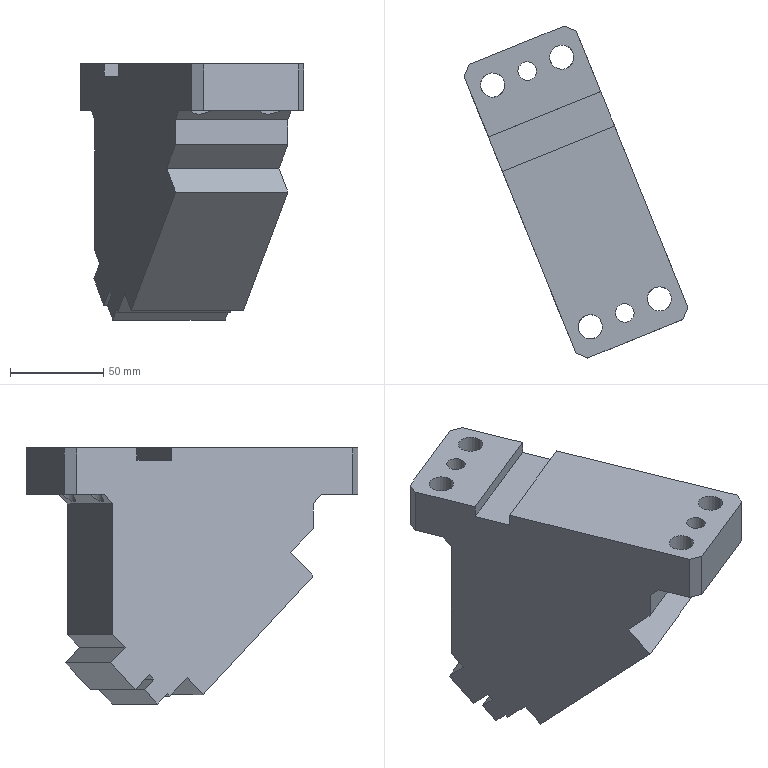Part | NX | features solid 2 | 1 solid | 47 faces | box 120.204 x 178.225 x 137.53 mm | volume 892519 mm3 | plane 37 | cylinder 10 | commonest cylinder face diameters 13 x4 20 x4 10 x2
STEP:
#1=CARTESIAN_POINT('',(-779.548,445.031,38.127));
#2=VERTEX_POINT('',#1);
#3=CARTESIAN_POINT('',(-719.281,469.38,38.127));
#4=VERTEX_POINT('',#3);
#5=CARTESIAN_POINT('',(-779.548,445.031,38.127));
#6=DIRECTION('',(0.9272,0.3746,0.));
#7=VECTOR('',#6,1000.);
#8=LINE('',#5,#7);
#9=EDGE_CURVE('',#2,#4,#8,.T.);
#10=ORIENTED_EDGE('',*,*,#9,.T.);
#11=CARTESIAN_POINT('',(-718.752,468.069,36.712));
#12=VERTEX_POINT('',#11);
#13=CARTESIAN_POINT('',(-731.128,498.702,69.751));
#14=DIRECTION('',(0.2649,-0.6556,-0.7071));
#15=VECTOR('',#14,1000.);
#16=LINE('',#13,#15);
#17=EDGE_CURVE('',#4,#12,#16,.T.);
#18=ORIENTED_EDGE('',*,*,#17,.T.);
#19=CARTESIAN_POINT('',(-779.018,443.719,36.712));
#20=VERTEX_POINT('',#19);
#21=CARTESIAN_POINT('',(-779.018,443.719,36.712));
#22=DIRECTION('',(0.9272,0.3746,0.));
#23=VECTOR('',#22,1000.);
#24=LINE('',#21,#23);
#25=EDGE_CURVE('',#20,#12,#24,.T.);
#26=ORIENTED_EDGE('',*,*,#25,.F.);
#27=CARTESIAN_POINT('',(-791.395,474.352,69.751));
#28=DIRECTION('',(0.2649,-0.6556,-0.7071));
#29=VECTOR('',#28,1000.);
#30=LINE('',#27,#29);
#31=EDGE_CURVE('',#2,#20,#30,.T.);
#32=ORIENTED_EDGE('',*,*,#31,.F.);
#33=EDGE_LOOP('',(#10,#18,#26,#32));
#34=FACE_BOUND('',#33,.T.);
#35=CARTESIAN_POINT('',(-791.395,474.352,69.751));
#36=DIRECTION('',(-0.2649,0.6556,-0.7071));
#37=DIRECTION('',(0.2649,-0.6556,-0.7071));
#38=AXIS2_PLACEMENT_3D('',#35,#36,#37);
#39=PLANE('',#38);
#40=ADVANCED_FACE('',(#34),#39,.T.);
#41=CARTESIAN_POINT('',(-791.395,474.352,69.751));
#42=VERTEX_POINT('',#41);
#43=CARTESIAN_POINT('',(-788.746,467.796,62.68));
#44=VERTEX_POINT('',#43);
#45=CARTESIAN_POINT('',(-791.395,474.352,69.751));
#46=DIRECTION('',(0.2649,-0.6556,-0.7071));
#47=VECTOR('',#46,1000.);
#48=LINE('',#45,#47);
#49=EDGE_CURVE('',#42,#44,#48,.T.);
#50=ORIENTED_EDGE('',*,*,#49,.F.);
#51=CARTESIAN_POINT('',(-731.128,498.702,69.751));
#52=VERTEX_POINT('',#51);
#53=CARTESIAN_POINT('',(-791.395,474.352,69.751));
#54=DIRECTION('',(0.9272,0.3746,0.));
#55=VECTOR('',#54,1000.);
#56=LINE('',#53,#55);
#57=EDGE_CURVE('',#42,#52,#56,.T.);
#58=ORIENTED_EDGE('',*,*,#57,.T.);
#59=CARTESIAN_POINT('',(-728.479,492.145,62.68));
#60=VERTEX_POINT('',#59);
#61=CARTESIAN_POINT('',(-731.128,498.702,69.751));
#62=DIRECTION('',(0.2649,-0.6556,-0.7071));
#63=VECTOR('',#62,1000.);
#64=LINE('',#61,#63);
#65=EDGE_CURVE('',#52,#60,#64,.T.);
#66=ORIENTED_EDGE('',*,*,#65,.T.);
#67=CARTESIAN_POINT('',(-788.746,467.796,62.68));
#68=DIRECTION('',(0.9272,0.3746,0.));
#69=VECTOR('',#68,1000.);
#70=LINE('',#67,#69);
#71=EDGE_CURVE('',#44,#60,#70,.T.);
#72=ORIENTED_EDGE('',*,*,#71,.F.);
#73=EDGE_LOOP('',(#50,#58,#66,#72));
#74=FACE_BOUND('',#73,.T.);
#75=CARTESIAN_POINT('',(-791.395,474.352,69.751));
#76=DIRECTION('',(-0.2649,0.6556,-0.7071));
#77=DIRECTION('',(0.2649,-0.6556,-0.7071));
#78=AXIS2_PLACEMENT_3D('',#75,#76,#77);
#79=PLANE('',#78);
#80=ADVANCED_FACE('',(#74),#79,.T.);
#81=CARTESIAN_POINT('',(-782.462,452.243,45.905));
#82=VERTEX_POINT('',#81);
#83=CARTESIAN_POINT('',(-722.195,476.592,45.905));
#84=VERTEX_POINT('',#83);
#85=CARTESIAN_POINT('',(-782.462,452.243,45.905));
#86=DIRECTION('',(0.9272,0.3746,0.));
#87=VECTOR('',#86,1000.);
#88=LINE('',#85,#87);
#89=EDGE_CURVE('',#82,#84,#88,.T.);
#90=ORIENTED_EDGE('',*,*,#89,.F.);
#91=CARTESIAN_POINT('',(-783.448,454.684,48.538));
#92=VERTEX_POINT('',#91);
#93=CARTESIAN_POINT('',(-791.395,474.352,69.751));
#94=DIRECTION('',(0.2649,-0.6556,-0.7071));
#95=VECTOR('',#94,1000.);
#96=LINE('',#93,#95);
#97=EDGE_CURVE('',#92,#82,#96,.T.);
#98=ORIENTED_EDGE('',*,*,#97,.F.);
#99=CARTESIAN_POINT('',(-723.181,479.033,48.538));
#100=VERTEX_POINT('',#99);
#101=CARTESIAN_POINT('',(-783.448,454.684,48.538));
#102=DIRECTION('',(0.9272,0.3746,0.));
#103=VECTOR('',#102,1000.);
#104=LINE('',#101,#103);
#105=EDGE_CURVE('',#92,#100,#104,.T.);
#106=ORIENTED_EDGE('',*,*,#105,.T.);
#107=CARTESIAN_POINT('',(-731.128,498.702,69.751));
#108=DIRECTION('',(0.2649,-0.6556,-0.7071));
#109=VECTOR('',#108,1000.);
#110=LINE('',#107,#109);
#111=EDGE_CURVE('',#100,#84,#110,.T.);
#112=ORIENTED_EDGE('',*,*,#111,.T.);
#113=EDGE_LOOP('',(#90,#98,#106,#112));
#114=FACE_BOUND('',#113,.T.);
#115=CARTESIAN_POINT('',(-791.395,474.352,69.751));
#116=DIRECTION('',(-0.2649,0.6556,-0.7071));
#117=DIRECTION('',(0.2649,-0.6556,-0.7071));
#118=AXIS2_PLACEMENT_3D('',#115,#116,#117);
#119=PLANE('',#118);
#120=ADVANCED_FACE('',(#114),#119,.T.);
#121=CARTESIAN_POINT('',(-714.987,458.751,46.763));
#122=VERTEX_POINT('',#121);
#123=CARTESIAN_POINT('',(-718.752,468.069,36.712));
#124=DIRECTION('',(0.2649,-0.6556,0.7071));
#125=VECTOR('',#124,1000.);
#126=LINE('',#123,#125);
#127=EDGE_CURVE('',#12,#122,#126,.T.);
#128=ORIENTED_EDGE('',*,*,#127,.T.);
#129=CARTESIAN_POINT('',(-775.254,434.401,46.763));
#130=VERTEX_POINT('',#129);
#131=CARTESIAN_POINT('',(-775.254,434.401,46.763));
#132=DIRECTION('',(0.9272,0.3746,0.));
#133=VECTOR('',#132,1000.);
#134=LINE('',#131,#133);
#135=EDGE_CURVE('',#130,#122,#134,.T.);
#136=ORIENTED_EDGE('',*,*,#135,.F.);
#137=CARTESIAN_POINT('',(-779.018,443.719,36.712));
#138=DIRECTION('',(0.2649,-0.6556,0.7071));
#139=VECTOR('',#138,1000.);
#140=LINE('',#137,#139);
#141=EDGE_CURVE('',#20,#130,#140,.T.);
#142=ORIENTED_EDGE('',*,*,#141,.F.);
#143=ORIENTED_EDGE('',*,*,#25,.T.);
#144=EDGE_LOOP('',(#128,#136,#142,#143));
#145=FACE_BOUND('',#144,.T.);
#146=CARTESIAN_POINT('',(-779.018,443.719,36.712));
#147=DIRECTION('',(0.2649,-0.6556,-0.7071));
#148=DIRECTION('',(0.2649,-0.6556,0.7071));
#149=AXIS2_PLACEMENT_3D('',#146,#147,#148);
#150=PLANE('',#149);
#151=ADVANCED_FACE('',(#145),#150,.T.);
#152=CARTESIAN_POINT('',(-711.543,450.228,37.57));
#153=VERTEX_POINT('',#152);
#154=CARTESIAN_POINT('',(-714.987,458.751,46.763));
#155=DIRECTION('',(0.2649,-0.6556,-0.7071));
#156=VECTOR('',#155,1000.);
#157=LINE('',#154,#156);
#158=EDGE_CURVE('',#122,#153,#157,.T.);
#159=ORIENTED_EDGE('',*,*,#158,.T.);
#160=CARTESIAN_POINT('',(-771.81,425.878,37.57));
#161=VERTEX_POINT('',#160);
#162=CARTESIAN_POINT('',(-771.81,425.878,37.57));
#163=DIRECTION('',(0.9272,0.3746,0.));
#164=VECTOR('',#163,1000.);
#165=LINE('',#162,#164);
#166=EDGE_CURVE('',#161,#153,#165,.T.);
#167=ORIENTED_EDGE('',*,*,#166,.F.);
#168=CARTESIAN_POINT('',(-775.254,434.401,46.763));
#169=DIRECTION('',(0.2649,-0.6556,-0.7071));
#170=VECTOR('',#169,1000.);
#171=LINE('',#168,#170);
#172=EDGE_CURVE('',#130,#161,#171,.T.);
#173=ORIENTED_EDGE('',*,*,#172,.F.);
#174=ORIENTED_EDGE('',*,*,#135,.T.);
#175=EDGE_LOOP('',(#159,#167,#173,#174));
#176=FACE_BOUND('',#175,.T.);
#177=CARTESIAN_POINT('',(-775.254,434.401,46.763));
#178=DIRECTION('',(-0.2649,0.6556,-0.7071));
#179=DIRECTION('',(0.2649,-0.6556,-0.7071));
#180=AXIS2_PLACEMENT_3D('',#177,#178,#179);
#181=PLANE('',#180);
#182=ADVANCED_FACE('',(#176),#181,.T.);
#183=CARTESIAN_POINT('',(-687.703,391.222,101.21));
#184=VERTEX_POINT('',#183);
#185=CARTESIAN_POINT('',(-711.543,450.228,37.57));
#186=DIRECTION('',(0.2649,-0.6556,0.7071));
#187=VECTOR('',#186,1000.);
#188=LINE('',#185,#187);
#189=EDGE_CURVE('',#153,#184,#188,.T.);
#190=ORIENTED_EDGE('',*,*,#189,.T.);
#191=CARTESIAN_POINT('',(-747.97,366.873,101.21));
#192=VERTEX_POINT('',#191);
#193=CARTESIAN_POINT('',(-747.97,366.873,101.21));
#194=DIRECTION('',(0.9272,0.3746,0.));
#195=VECTOR('',#194,1000.);
#196=LINE('',#193,#195);
#197=EDGE_CURVE('',#192,#184,#196,.T.);
#198=ORIENTED_EDGE('',*,*,#197,.F.);
#199=CARTESIAN_POINT('',(-771.81,425.878,37.57));
#200=DIRECTION('',(0.2649,-0.6556,0.7071));
#201=VECTOR('',#200,1000.);
#202=LINE('',#199,#201);
#203=EDGE_CURVE('',#161,#192,#202,.T.);
#204=ORIENTED_EDGE('',*,*,#203,.F.);
#205=ORIENTED_EDGE('',*,*,#166,.T.);
#206=EDGE_LOOP('',(#190,#198,#204,#205));
#207=FACE_BOUND('',#206,.T.);
#208=CARTESIAN_POINT('',(-771.81,425.878,37.57));
#209=DIRECTION('',(0.2649,-0.6556,-0.7071));
#210=DIRECTION('',(0.2649,-0.6556,0.7071));
#211=AXIS2_PLACEMENT_3D('',#208,#209,#210);
#212=PLANE('',#211);
#213=ADVANCED_FACE('',(#207),#212,.T.);
#214=CARTESIAN_POINT('',(-692.471,403.023,113.938));
#215=VERTEX_POINT('',#214);
#216=CARTESIAN_POINT('',(-692.471,403.023,113.938));
#217=DIRECTION('',(0.2649,-0.6556,-0.7071));
#218=VECTOR('',#217,1000.);
#219=LINE('',#216,#218);
#220=EDGE_CURVE('',#215,#184,#219,.T.);
#221=ORIENTED_EDGE('',*,*,#220,.F.);
#222=CARTESIAN_POINT('',(-752.738,378.674,113.938));
#223=VERTEX_POINT('',#222);
#224=CARTESIAN_POINT('',(-752.738,378.674,113.938));
#225=DIRECTION('',(0.9272,0.3746,0.));
#226=VECTOR('',#225,1000.);
#227=LINE('',#224,#226);
#228=EDGE_CURVE('',#223,#215,#227,.T.);
#229=ORIENTED_EDGE('',*,*,#228,.F.);
#230=CARTESIAN_POINT('',(-752.738,378.674,113.938));
#231=DIRECTION('',(0.2649,-0.6556,-0.7071));
#232=VECTOR('',#231,1000.);
#233=LINE('',#230,#232);
#234=EDGE_CURVE('',#223,#192,#233,.T.);
#235=ORIENTED_EDGE('',*,*,#234,.T.);
#236=ORIENTED_EDGE('',*,*,#197,.T.);
#237=EDGE_LOOP('',(#221,#229,#235,#236));
#238=FACE_BOUND('',#237,.T.);
#239=CARTESIAN_POINT('',(-752.738,378.674,113.938));
#240=DIRECTION('',(-0.2649,0.6556,-0.7071));
#241=DIRECTION('',(0.2649,-0.6556,-0.7071));
#242=AXIS2_PLACEMENT_3D('',#239,#240,#241);
#243=PLANE('',#242);
#244=ADVANCED_FACE('',(#238),#243,.F.);
#245=CARTESIAN_POINT('',(-687.674,391.148,126.745));
#246=VERTEX_POINT('',#245);
#247=CARTESIAN_POINT('',(-692.471,403.023,113.938));
#248=DIRECTION('',(0.2649,-0.6556,0.7071));
#249=VECTOR('',#248,1000.);
#250=LINE('',#247,#249);
#251=EDGE_CURVE('',#215,#246,#250,.T.);
#252=ORIENTED_EDGE('',*,*,#251,.T.);
#253=CARTESIAN_POINT('',(-747.941,366.799,126.745));
#254=VERTEX_POINT('',#253);
#255=CARTESIAN_POINT('',(-747.941,366.799,126.745));
#256=DIRECTION('',(0.9272,0.3746,0.));
#257=VECTOR('',#256,1000.);
#258=LINE('',#255,#257);
#259=EDGE_CURVE('',#254,#246,#258,.T.);
#260=ORIENTED_EDGE('',*,*,#259,.F.);
#261=CARTESIAN_POINT('',(-752.738,378.674,113.938));
#262=DIRECTION('',(0.2649,-0.6556,0.7071));
#263=VECTOR('',#262,1000.);
#264=LINE('',#261,#263);
#265=EDGE_CURVE('',#223,#254,#264,.T.);
#266=ORIENTED_EDGE('',*,*,#265,.F.);
#267=ORIENTED_EDGE('',*,*,#228,.T.);
#268=EDGE_LOOP('',(#252,#260,#266,#267));
#269=FACE_BOUND('',#268,.T.);
#270=CARTESIAN_POINT('',(-752.738,378.674,113.938));
#271=DIRECTION('',(0.2649,-0.6556,-0.7071));
#272=DIRECTION('',(0.2649,-0.6556,0.7071));
#273=AXIS2_PLACEMENT_3D('',#270,#271,#272);
#274=PLANE('',#273);
#275=ADVANCED_FACE('',(#269),#274,.T.);
#276=CARTESIAN_POINT('',(-747.941,366.799,140.));
#277=VERTEX_POINT('',#276);
#278=CARTESIAN_POINT('',(-747.941,366.799,145.));
#279=DIRECTION('',(0.,0.,-1.));
#280=VECTOR('',#279,1000.);
#281=LINE('',#278,#280);
#282=EDGE_CURVE('',#277,#254,#281,.T.);
#283=ORIENTED_EDGE('',*,*,#282,.T.);
#284=ORIENTED_EDGE('',*,*,#259,.T.);
#285=CARTESIAN_POINT('',(-687.674,391.148,140.));
#286=VERTEX_POINT('',#285);
#287=CARTESIAN_POINT('',(-687.674,391.148,145.));
#288=DIRECTION('',(0.,0.,-1.));
#289=VECTOR('',#288,1000.);
#290=LINE('',#287,#289);
#291=EDGE_CURVE('',#286,#246,#290,.T.);
#292=ORIENTED_EDGE('',*,*,#291,.F.);
#293=CARTESIAN_POINT('',(-747.941,366.799,140.));
#294=DIRECTION('',(0.9272,0.3746,0.));
#295=VECTOR('',#294,1000.);
#296=LINE('',#293,#295);
#297=EDGE_CURVE('',#277,#286,#296,.T.);
#298=ORIENTED_EDGE('',*,*,#297,.F.);
#299=EDGE_LOOP('',(#283,#284,#292,#298));
#300=FACE_BOUND('',#299,.T.);
#301=CARTESIAN_POINT('',(-747.941,366.799,145.));
#302=DIRECTION('',(-0.3746,0.9272,0.));
#303=DIRECTION('',(0.9272,0.3746,0.));
#304=AXIS2_PLACEMENT_3D('',#301,#302,#303);
#305=PLANE('',#304);
#306=ADVANCED_FACE('',(#300),#305,.F.);
#307=CARTESIAN_POINT('',(-731.128,498.702,140.));
#308=VERTEX_POINT('',#307);
#309=CARTESIAN_POINT('',(-731.128,498.702,69.751));
#310=DIRECTION('',(0.,0.,1.));
#311=VECTOR('',#310,1000.);
#312=LINE('',#309,#311);
#313=EDGE_CURVE('',#52,#308,#312,.T.);
#314=ORIENTED_EDGE('',*,*,#313,.F.);
#315=ORIENTED_EDGE('',*,*,#57,.F.);
#316=CARTESIAN_POINT('',(-791.395,474.352,140.));
#317=VERTEX_POINT('',#316);
#318=CARTESIAN_POINT('',(-791.395,474.352,69.751));
#319=DIRECTION('',(0.,0.,1.));
#320=VECTOR('',#319,1000.);
#321=LINE('',#318,#320);
#322=EDGE_CURVE('',#42,#317,#321,.T.);
#323=ORIENTED_EDGE('',*,*,#322,.T.);
#324=CARTESIAN_POINT('',(-791.395,474.352,140.));
#325=DIRECTION('',(-0.9272,-0.3746,0.));
#326=VECTOR('',#325,1000.);
#327=LINE('',#324,#326);
#328=EDGE_CURVE('',#308,#317,#327,.T.);
#329=ORIENTED_EDGE('',*,*,#328,.F.);
#330=EDGE_LOOP('',(#314,#315,#323,#329));
#331=FACE_BOUND('',#330,.T.);
#332=CARTESIAN_POINT('',(-791.395,474.352,69.751));
#333=DIRECTION('',(0.3746,-0.9272,0.));
#334=DIRECTION('',(-0.9272,-0.3746,0.));
#335=AXIS2_PLACEMENT_3D('',#332,#333,#334);
#336=PLANE('',#335);
#337=ADVANCED_FACE('',(#331),#336,.F.);
#338=CARTESIAN_POINT('',(-778.658,442.828,170.));
#339=VERTEX_POINT('',#338);
#340=CARTESIAN_POINT('',(-739.325,345.474,170.));
#341=VERTEX_POINT('',#340);
#342=CARTESIAN_POINT('',(-801.135,498.459,170.));
#343=DIRECTION('',(0.3746,-0.9272,0.));
#344=VECTOR('',#343,1000.);
#345=LINE('',#342,#344);
#346=EDGE_CURVE('',#339,#341,#345,.T.);
#347=ORIENTED_EDGE('',*,*,#346,.F.);
#348=CARTESIAN_POINT('',(-778.658,442.828,163.5));
#349=VERTEX_POINT('',#348);
#350=CARTESIAN_POINT('',(-778.658,442.828,163.5));
#351=DIRECTION('',(0.,0.,1.));
#352=VECTOR('',#351,1000.);
#353=LINE('',#350,#352);
#354=EDGE_CURVE('',#349,#339,#353,.T.);
#355=ORIENTED_EDGE('',*,*,#354,.F.);
#356=CARTESIAN_POINT('',(-786.15,461.372,163.5));
#357=VERTEX_POINT('',#356);
#358=CARTESIAN_POINT('',(-786.15,461.372,163.5));
#359=DIRECTION('',(0.3746,-0.9272,0.));
#360=VECTOR('',#359,1000.);
#361=LINE('',#358,#360);
#362=EDGE_CURVE('',#357,#349,#361,.T.);
#363=ORIENTED_EDGE('',*,*,#362,.F.);
#364=CARTESIAN_POINT('',(-786.15,461.372,170.));
#365=VERTEX_POINT('',#364);
#366=CARTESIAN_POINT('',(-786.15,461.372,170.));
#367=DIRECTION('',(0.,0.,-1.));
#368=VECTOR('',#367,1000.);
#369=LINE('',#366,#368);
#370=EDGE_CURVE('',#365,#357,#369,.T.);
#371=ORIENTED_EDGE('',*,*,#370,.F.);
#372=CARTESIAN_POINT('',(-799.262,493.823,170.));
#373=VERTEX_POINT('',#372);
#374=CARTESIAN_POINT('',(-801.135,498.459,170.));
#375=DIRECTION('',(0.3746,-0.9272,0.));
#376=VECTOR('',#375,1000.);
#377=LINE('',#374,#376);
#378=EDGE_CURVE('',#373,#365,#377,.T.);
#379=ORIENTED_EDGE('',*,*,#378,.F.);
#380=CARTESIAN_POINT('',(-799.262,493.823,145.));
#381=VERTEX_POINT('',#380);
#382=CARTESIAN_POINT('',(-799.262,493.823,27.52));
#383=DIRECTION('',(0.,0.,1.));
#384=VECTOR('',#383,1000.);
#385=LINE('',#382,#384);
#386=EDGE_CURVE('',#381,#373,#385,.T.);
#387=ORIENTED_EDGE('',*,*,#386,.F.);
#388=CARTESIAN_POINT('',(-793.268,478.988,145.));
#389=VERTEX_POINT('',#388);
#390=CARTESIAN_POINT('',(-801.135,498.459,145.));
#391=DIRECTION('',(0.3746,-0.9272,0.));
#392=VECTOR('',#391,1000.);
#393=LINE('',#390,#392);
#394=EDGE_CURVE('',#381,#389,#393,.T.);
#395=ORIENTED_EDGE('',*,*,#394,.T.);
#396=CARTESIAN_POINT('',(-762.417,402.63,62.645));
#397=DIRECTION('',(-0.2649,0.6556,0.7071));
#398=VECTOR('',#397,1000.);
#399=LINE('',#396,#398);
#400=EDGE_CURVE('',#317,#389,#399,.T.);
#401=ORIENTED_EDGE('',*,*,#400,.F.);
#402=ORIENTED_EDGE('',*,*,#322,.F.);
#403=ORIENTED_EDGE('',*,*,#49,.T.);
#404=CARTESIAN_POINT('',(-791.792,475.336,54.548));
#405=VERTEX_POINT('',#404);
#406=CARTESIAN_POINT('',(-788.746,467.796,62.68));
#407=DIRECTION('',(-0.2649,0.6556,-0.7071));
#408=VECTOR('',#407,1000.);
#409=LINE('',#406,#408);
#410=EDGE_CURVE('',#405,#44,#409,.F.);
#411=ORIENTED_EDGE('',*,*,#410,.F.);
#412=CARTESIAN_POINT('',(-786.494,462.223,40.406));
#413=VERTEX_POINT('',#412);
#414=CARTESIAN_POINT('',(-786.494,462.223,40.406));
#415=DIRECTION('',(0.2649,-0.6556,-0.7071));
#416=VECTOR('',#415,1000.);
#417=LINE('',#414,#416);
#418=EDGE_CURVE('',#413,#405,#417,.F.);
#419=ORIENTED_EDGE('',*,*,#418,.F.);
#420=CARTESIAN_POINT('',(-783.448,454.684,48.538));
#421=DIRECTION('',(-0.2649,0.6556,-0.7071));
#422=VECTOR('',#421,1000.);
#423=LINE('',#420,#422);
#424=EDGE_CURVE('',#413,#92,#423,.F.);
#425=ORIENTED_EDGE('',*,*,#424,.T.);
#426=ORIENTED_EDGE('',*,*,#97,.T.);
#427=CARTESIAN_POINT('',(-784.581,457.487,40.248));
#428=VERTEX_POINT('',#427);
#429=CARTESIAN_POINT('',(-782.462,452.243,45.905));
#430=DIRECTION('',(0.2649,-0.6556,0.7071));
#431=VECTOR('',#430,1000.);
#432=LINE('',#429,#431);
#433=EDGE_CURVE('',#428,#82,#432,.T.);
#434=ORIENTED_EDGE('',*,*,#433,.F.);
#435=CARTESIAN_POINT('',(-781.667,450.276,32.47));
#436=VERTEX_POINT('',#435);
#437=CARTESIAN_POINT('',(-781.667,450.276,32.47));
#438=DIRECTION('',(0.2649,-0.6556,-0.7071));
#439=VECTOR('',#438,1000.);
#440=LINE('',#437,#439);
#441=EDGE_CURVE('',#436,#428,#440,.F.);
#442=ORIENTED_EDGE('',*,*,#441,.F.);
#443=CARTESIAN_POINT('',(-779.548,445.031,38.127));
#444=DIRECTION('',(0.2649,-0.6556,0.7071));
#445=VECTOR('',#444,1000.);
#446=LINE('',#443,#445);
#447=EDGE_CURVE('',#436,#2,#446,.T.);
#448=ORIENTED_EDGE('',*,*,#447,.T.);
#449=ORIENTED_EDGE('',*,*,#31,.T.);
#450=ORIENTED_EDGE('',*,*,#141,.T.);
#451=ORIENTED_EDGE('',*,*,#172,.T.);
#452=ORIENTED_EDGE('',*,*,#203,.T.);
#453=ORIENTED_EDGE('',*,*,#234,.F.);
#454=ORIENTED_EDGE('',*,*,#265,.T.);
#455=ORIENTED_EDGE('',*,*,#282,.F.);
#456=CARTESIAN_POINT('',(-746.067,362.163,145.));
#457=VERTEX_POINT('',#456);
#458=CARTESIAN_POINT('',(-782.826,453.142,46.875));
#459=DIRECTION('',(-0.2649,0.6556,-0.7071));
#460=VECTOR('',#459,1000.);
#461=LINE('',#458,#460);
#462=EDGE_CURVE('',#457,#277,#461,.T.);
#463=ORIENTED_EDGE('',*,*,#462,.F.);
#464=CARTESIAN_POINT('',(-739.325,345.474,145.));
#465=VERTEX_POINT('',#464);
#466=CARTESIAN_POINT('',(-801.135,498.459,145.));
#467=DIRECTION('',(0.3746,-0.9272,0.));
#468=VECTOR('',#467,1000.);
#469=LINE('',#466,#468);
#470=EDGE_CURVE('',#457,#465,#469,.T.);
#471=ORIENTED_EDGE('',*,*,#470,.T.);
#472=CARTESIAN_POINT('',(-739.325,345.474,145.));
#473=DIRECTION('',(0.,0.,-1.));
#474=VECTOR('',#473,1000.);
#475=LINE('',#472,#474);
#476=EDGE_CURVE('',#341,#465,#475,.T.);
#477=ORIENTED_EDGE('',*,*,#476,.F.);
#478=EDGE_LOOP('',(#347,#355,#363,#371,#379,#387,#395,#401,#402,#403,#411,#419,#425,#426,#434,#442,#448,#449,#450,#451,#452,#453,#454,#455,#463,#471,#477));
#479=FACE_BOUND('',#478,.T.);
#480=CARTESIAN_POINT('',(-775.575,435.196,27.52));
#481=DIRECTION('',(0.9272,0.3746,0.));
#482=DIRECTION('',(0.3746,-0.9272,0.));
#483=AXIS2_PLACEMENT_3D('',#480,#481,#482);
#484=PLANE('',#483);
#485=ADVANCED_FACE('',(#479),#484,.F.);
#486=ORIENTED_EDGE('',*,*,#291,.T.);
#487=ORIENTED_EDGE('',*,*,#251,.F.);
#488=ORIENTED_EDGE('',*,*,#220,.T.);
#489=ORIENTED_EDGE('',*,*,#189,.F.);
#490=ORIENTED_EDGE('',*,*,#158,.F.);
#491=ORIENTED_EDGE('',*,*,#127,.F.);
#492=ORIENTED_EDGE('',*,*,#17,.F.);
#493=CARTESIAN_POINT('',(-721.4,474.625,32.47));
#494=VERTEX_POINT('',#493);
#495=CARTESIAN_POINT('',(-719.281,469.38,38.127));
#496=DIRECTION('',(0.2649,-0.6556,0.7071));
#497=VECTOR('',#496,1000.);
#498=LINE('',#495,#497);
#499=EDGE_CURVE('',#494,#4,#498,.T.);
#500=ORIENTED_EDGE('',*,*,#499,.F.);
#501=CARTESIAN_POINT('',(-724.314,481.837,40.248));
#502=VERTEX_POINT('',#501);
#503=CARTESIAN_POINT('',(-721.4,474.625,32.47));
#504=DIRECTION('',(0.2649,-0.6556,-0.7071));
#505=VECTOR('',#504,1000.);
#506=LINE('',#503,#505);
#507=EDGE_CURVE('',#494,#502,#506,.F.);
#508=ORIENTED_EDGE('',*,*,#507,.T.);
#509=CARTESIAN_POINT('',(-722.195,476.592,45.905));
#510=DIRECTION('',(0.2649,-0.6556,0.7071));
#511=VECTOR('',#510,1000.);
#512=LINE('',#509,#511);
#513=EDGE_CURVE('',#502,#84,#512,.T.);
#514=ORIENTED_EDGE('',*,*,#513,.T.);
#515=ORIENTED_EDGE('',*,*,#111,.F.);
#516=CARTESIAN_POINT('',(-726.228,486.573,40.406));
#517=VERTEX_POINT('',#516);
#518=CARTESIAN_POINT('',(-723.181,479.033,48.538));
#519=DIRECTION('',(-0.2649,0.6556,-0.7071));
#520=VECTOR('',#519,1000.);
#521=LINE('',#518,#520);
#522=EDGE_CURVE('',#517,#100,#521,.F.);
#523=ORIENTED_EDGE('',*,*,#522,.F.);
#524=CARTESIAN_POINT('',(-731.525,499.685,54.548));
#525=VERTEX_POINT('',#524);
#526=CARTESIAN_POINT('',(-726.228,486.573,40.406));
#527=DIRECTION('',(0.2649,-0.6556,-0.7071));
#528=VECTOR('',#527,1000.);
#529=LINE('',#526,#528);
#530=EDGE_CURVE('',#517,#525,#529,.F.);
#531=ORIENTED_EDGE('',*,*,#530,.T.);
#532=CARTESIAN_POINT('',(-728.479,492.145,62.68));
#533=DIRECTION('',(-0.2649,0.6556,-0.7071));
#534=VECTOR('',#533,1000.);
#535=LINE('',#532,#534);
#536=EDGE_CURVE('',#525,#60,#535,.F.);
#537=ORIENTED_EDGE('',*,*,#536,.T.);
#538=ORIENTED_EDGE('',*,*,#65,.F.);
#539=ORIENTED_EDGE('',*,*,#313,.T.);
#540=CARTESIAN_POINT('',(-733.001,503.338,145.));
#541=VERTEX_POINT('',#540);
#542=CARTESIAN_POINT('',(-733.001,503.338,145.));
#543=DIRECTION('',(0.2649,-0.6556,-0.7071));
#544=VECTOR('',#543,1000.);
#545=LINE('',#542,#544);
#546=EDGE_CURVE('',#541,#308,#545,.T.);
#547=ORIENTED_EDGE('',*,*,#546,.F.);
#548=CARTESIAN_POINT('',(-738.995,518.173,145.));
#549=VERTEX_POINT('',#548);
#550=CARTESIAN_POINT('',(-740.868,522.808,145.));
#551=DIRECTION('',(0.3746,-0.9272,0.));
#552=VECTOR('',#551,1000.);
#553=LINE('',#550,#552);
#554=EDGE_CURVE('',#549,#541,#553,.T.);
#555=ORIENTED_EDGE('',*,*,#554,.F.);
#556=CARTESIAN_POINT('',(-738.995,518.173,170.));
#557=VERTEX_POINT('',#556);
#558=CARTESIAN_POINT('',(-738.995,518.173,145.));
#559=DIRECTION('',(0.,0.,-1.));
#560=VECTOR('',#559,1000.);
#561=LINE('',#558,#560);
#562=EDGE_CURVE('',#557,#549,#561,.T.);
#563=ORIENTED_EDGE('',*,*,#562,.F.);
#564=CARTESIAN_POINT('',(-725.883,485.721,170.));
#565=VERTEX_POINT('',#564);
#566=CARTESIAN_POINT('',(-740.868,522.808,170.));
#567=DIRECTION('',(0.3746,-0.9272,0.));
#568=VECTOR('',#567,1000.);
#569=LINE('',#566,#568);
#570=EDGE_CURVE('',#557,#565,#569,.T.);
#571=ORIENTED_EDGE('',*,*,#570,.T.);
#572=CARTESIAN_POINT('',(-725.883,485.721,163.5));
#573=VERTEX_POINT('',#572);
#574=CARTESIAN_POINT('',(-725.883,485.721,170.));
#575=DIRECTION('',(0.,0.,-1.));
#576=VECTOR('',#575,1000.);
#577=LINE('',#574,#576);
#578=EDGE_CURVE('',#565,#573,#577,.T.);
#579=ORIENTED_EDGE('',*,*,#578,.T.);
#580=CARTESIAN_POINT('',(-718.391,467.177,163.5));
#581=VERTEX_POINT('',#580);
#582=CARTESIAN_POINT('',(-725.883,485.721,163.5));
#583=DIRECTION('',(0.3746,-0.9272,0.));
#584=VECTOR('',#583,1000.);
#585=LINE('',#582,#584);
#586=EDGE_CURVE('',#573,#581,#585,.T.);
#587=ORIENTED_EDGE('',*,*,#586,.T.);
#588=CARTESIAN_POINT('',(-718.391,467.177,170.));
#589=VERTEX_POINT('',#588);
#590=CARTESIAN_POINT('',(-718.391,467.177,163.5));
#591=DIRECTION('',(0.,0.,1.));
#592=VECTOR('',#591,1000.);
#593=LINE('',#590,#592);
#594=EDGE_CURVE('',#581,#589,#593,.T.);
#595=ORIENTED_EDGE('',*,*,#594,.T.);
#596=CARTESIAN_POINT('',(-679.058,369.823,170.));
#597=VERTEX_POINT('',#596);
#598=CARTESIAN_POINT('',(-740.868,522.808,170.));
#599=DIRECTION('',(0.3746,-0.9272,0.));
#600=VECTOR('',#599,1000.);
#601=LINE('',#598,#600);
#602=EDGE_CURVE('',#589,#597,#601,.T.);
#603=ORIENTED_EDGE('',*,*,#602,.T.);
#604=CARTESIAN_POINT('',(-679.058,369.823,145.));
#605=VERTEX_POINT('',#604);
#606=CARTESIAN_POINT('',(-679.058,369.823,27.52));
#607=DIRECTION('',(0.,0.,1.));
#608=VECTOR('',#607,1000.);
#609=LINE('',#606,#608);
#610=EDGE_CURVE('',#605,#597,#609,.T.);
#611=ORIENTED_EDGE('',*,*,#610,.F.);
#612=CARTESIAN_POINT('',(-685.801,386.512,145.));
#613=VERTEX_POINT('',#612);
#614=CARTESIAN_POINT('',(-740.868,522.808,145.));
#615=DIRECTION('',(0.3746,-0.9272,0.));
#616=VECTOR('',#615,1000.);
#617=LINE('',#614,#616);
#618=EDGE_CURVE('',#613,#605,#617,.T.);
#619=ORIENTED_EDGE('',*,*,#618,.F.);
#620=CARTESIAN_POINT('',(-687.674,391.148,140.));
#621=DIRECTION('',(0.2649,-0.6556,0.7071));
#622=VECTOR('',#621,1000.);
#623=LINE('',#620,#622);
#624=EDGE_CURVE('',#286,#613,#623,.T.);
#625=ORIENTED_EDGE('',*,*,#624,.F.);
#626=EDGE_LOOP('',(#486,#487,#488,#489,#490,#491,#492,#500,#508,#514,#515,#523,#531,#537,#538,#539,#547,#555,#563,#571,#579,#587,#595,#603,#611,#619,#625));
#627=FACE_BOUND('',#626,.T.);
#628=CARTESIAN_POINT('',(-715.308,459.546,27.52));
#629=DIRECTION('',(0.9272,0.3746,0.));
#630=DIRECTION('',(0.3746,-0.9272,0.));
#631=AXIS2_PLACEMENT_3D('',#628,#629,#630);
#632=PLANE('',#631);
#633=ADVANCED_FACE('',(#627),#632,.T.);
#634=ORIENTED_EDGE('',*,*,#618,.T.);
#635=CARTESIAN_POINT('',(-681.821,363.314,145.));
#636=VERTEX_POINT('',#635);
#637=CARTESIAN_POINT('',(-651.429,434.913,145.));
#638=DIRECTION('',(-0.3907,-0.9205,0.));
#639=VECTOR('',#638,1000.);
#640=LINE('',#637,#639);
#641=EDGE_CURVE('',#636,#605,#640,.F.);
#642=ORIENTED_EDGE('',*,*,#641,.F.);
#643=CARTESIAN_POINT('',(-732.816,342.711,145.));
#644=VERTEX_POINT('',#643);
#645=CARTESIAN_POINT('',(-677.185,365.187,145.));
#646=DIRECTION('',(-0.9272,-0.3746,0.));
#647=VECTOR('',#646,1000.);
#648=LINE('',#645,#647);
#649=EDGE_CURVE('',#636,#644,#648,.T.);
#650=ORIENTED_EDGE('',*,*,#649,.T.);
#651=CARTESIAN_POINT('',(-846.722,391.061,145.));
#652=DIRECTION('',(0.9205,-0.3907,0.));
#653=VECTOR('',#652,1000.);
#654=LINE('',#651,#653);
#655=EDGE_CURVE('',#465,#644,#654,.T.);
#656=ORIENTED_EDGE('',*,*,#655,.F.);
#657=ORIENTED_EDGE('',*,*,#470,.F.);
#658=CARTESIAN_POINT('',(-740.041,364.598,145.));
#659=VERTEX_POINT('',#658);
#660=CARTESIAN_POINT('',(-746.067,362.163,145.));
#661=DIRECTION('',(-0.9272,-0.3746,0.));
#662=VECTOR('',#661,1000.);
#663=LINE('',#660,#662);
#664=EDGE_CURVE('',#659,#457,#663,.T.);
#665=ORIENTED_EDGE('',*,*,#664,.F.);
#666=CARTESIAN_POINT('',(-728.915,369.093,145.));
#667=VERTEX_POINT('',#666);
#668=CARTESIAN_POINT('',(-731.481,359.428,145.));
#669=DIRECTION('',(0.,0.,-1.));
#670=DIRECTION('',(0.3746,-0.9272,0.));
#671=AXIS2_PLACEMENT_3D('',#668,#669,#670);
#672=CIRCLE('',#671,10.);
#673=EDGE_CURVE('',#667,#659,#672,.T.);
#674=ORIENTED_EDGE('',*,*,#673,.F.);
#675=CARTESIAN_POINT('',(-702.953,379.582,145.));
#676=VERTEX_POINT('',#675);
#677=CARTESIAN_POINT('',(-746.067,362.163,145.));
#678=DIRECTION('',(-0.9272,-0.3746,0.));
#679=VECTOR('',#678,1000.);
#680=LINE('',#677,#679);
#681=EDGE_CURVE('',#676,#667,#680,.T.);
#682=ORIENTED_EDGE('',*,*,#681,.F.);
#683=CARTESIAN_POINT('',(-691.827,384.077,145.));
#684=VERTEX_POINT('',#683);
#685=CARTESIAN_POINT('',(-694.393,374.412,145.));
#686=DIRECTION('',(0.,0.,-1.));
#687=DIRECTION('',(0.3746,-0.9272,0.));
#688=AXIS2_PLACEMENT_3D('',#685,#686,#687);
#689=CIRCLE('',#688,10.);
#690=EDGE_CURVE('',#684,#676,#689,.T.);
#691=ORIENTED_EDGE('',*,*,#690,.F.);
#692=CARTESIAN_POINT('',(-746.067,362.163,145.));
#693=DIRECTION('',(-0.9272,-0.3746,0.));
#694=VECTOR('',#693,1000.);
#695=LINE('',#692,#694);
#696=EDGE_CURVE('',#613,#684,#695,.T.);
#697=ORIENTED_EDGE('',*,*,#696,.F.);
#698=EDGE_LOOP('',(#634,#642,#650,#656,#657,#665,#674,#682,#691,#697));
#699=FACE_BOUND('',#698,.T.);
#700=CARTESIAN_POINT('',(-711.064,362.284,145.));
#701=VERTEX_POINT('',#700);
#702=CARTESIAN_POINT('',(-712.937,366.92,145.));
#703=DIRECTION('',(0.,0.,-1.));
#704=DIRECTION('',(0.3746,-0.9272,0.));
#705=AXIS2_PLACEMENT_3D('',#702,#703,#704);
#706=CIRCLE('',#705,5.);
#707=EDGE_CURVE('',#701,#701,#706,.T.);
#708=ORIENTED_EDGE('',*,*,#707,.F.);
#709=EDGE_LOOP('',(#708));
#710=FACE_BOUND('',#709,.T.);
#711=CARTESIAN_POINT('',(-801.135,498.459,145.));
#712=DIRECTION('',(0.,0.,-1.));
#713=DIRECTION('',(-0.9272,-0.3746,0.));
#714=AXIS2_PLACEMENT_3D('',#711,#712,#713);
#715=PLANE('',#714);
#716=ADVANCED_FACE('',(#699,#710),#715,.T.);
#717=CARTESIAN_POINT('',(-691.959,368.386,170.));
#718=VERTEX_POINT('',#717);
#719=CARTESIAN_POINT('',(-694.393,374.412,170.));
#720=DIRECTION('',(0.,0.,-1.));
#721=DIRECTION('',(0.3746,-0.9272,0.));
#722=AXIS2_PLACEMENT_3D('',#719,#720,#721);
#723=CIRCLE('',#722,6.5);
#724=EDGE_CURVE('',#718,#718,#723,.T.);
#725=ORIENTED_EDGE('',*,*,#724,.T.);
#726=EDGE_LOOP('',(#725));
#727=FACE_BOUND('',#726,.T.);
#728=CARTESIAN_POINT('',(-711.064,362.284,170.));
#729=VERTEX_POINT('',#728);
#730=CARTESIAN_POINT('',(-712.937,366.92,170.));
#731=DIRECTION('',(0.,0.,-1.));
#732=DIRECTION('',(0.3746,-0.9272,0.));
#733=AXIS2_PLACEMENT_3D('',#730,#731,#732);
#734=CIRCLE('',#733,5.);
#735=EDGE_CURVE('',#729,#729,#734,.T.);
#736=ORIENTED_EDGE('',*,*,#735,.T.);
#737=EDGE_LOOP('',(#736));
#738=FACE_BOUND('',#737,.T.);
#739=CARTESIAN_POINT('',(-729.046,353.401,170.));
#740=VERTEX_POINT('',#739);
#741=CARTESIAN_POINT('',(-731.481,359.428,170.));
#742=DIRECTION('',(0.,0.,-1.));
#743=DIRECTION('',(0.3746,-0.9272,0.));
#744=AXIS2_PLACEMENT_3D('',#741,#742,#743);
#745=CIRCLE('',#744,6.5);
#746=EDGE_CURVE('',#740,#740,#745,.T.);
#747=ORIENTED_EDGE('',*,*,#746,.T.);
#748=EDGE_LOOP('',(#747));
#749=FACE_BOUND('',#748,.T.);
#750=CARTESIAN_POINT('',(-681.821,363.314,170.));
#751=VERTEX_POINT('',#750);
#752=CARTESIAN_POINT('',(-732.816,342.711,170.));
#753=VERTEX_POINT('',#752);
#754=CARTESIAN_POINT('',(-677.185,365.187,170.));
#755=DIRECTION('',(-0.9272,-0.3746,0.));
#756=VECTOR('',#755,1000.);
#757=LINE('',#754,#756);
#758=EDGE_CURVE('',#751,#753,#757,.T.);
#759=ORIENTED_EDGE('',*,*,#758,.F.);
#760=CARTESIAN_POINT('',(-679.058,369.823,170.));
#761=DIRECTION('',(0.3907,0.9205,0.));
#762=VECTOR('',#761,1000.);
#763=LINE('',#760,#762);
#764=EDGE_CURVE('',#597,#751,#763,.F.);
#765=ORIENTED_EDGE('',*,*,#764,.F.);
#766=ORIENTED_EDGE('',*,*,#602,.F.);
#767=CARTESIAN_POINT('',(-778.658,442.828,170.));
#768=DIRECTION('',(0.9272,0.3746,0.));
#769=VECTOR('',#768,1000.);
#770=LINE('',#767,#769);
#771=EDGE_CURVE('',#339,#589,#770,.T.);
#772=ORIENTED_EDGE('',*,*,#771,.F.);
#773=ORIENTED_EDGE('',*,*,#346,.T.);
#774=CARTESIAN_POINT('',(-732.816,342.711,170.));
#775=DIRECTION('',(-0.9205,0.3907,0.));
#776=VECTOR('',#775,1000.);
#777=LINE('',#774,#776);
#778=EDGE_CURVE('',#753,#341,#777,.T.);
#779=ORIENTED_EDGE('',*,*,#778,.F.);
#780=EDGE_LOOP('',(#759,#765,#766,#772,#773,#779));
#781=FACE_BOUND('',#780,.T.);
#782=CARTESIAN_POINT('',(-801.135,498.459,170.));
#783=DIRECTION('',(0.,0.,-1.));
#784=DIRECTION('',(-0.9272,-0.3746,0.));
#785=AXIS2_PLACEMENT_3D('',#782,#783,#784);
#786=PLANE('',#785);
#787=ADVANCED_FACE('',(#727,#738,#749,#781),#786,.F.);
#788=CARTESIAN_POINT('',(-745.504,520.935,170.));
#789=VERTEX_POINT('',#788);
#790=CARTESIAN_POINT('',(-796.499,500.332,170.));
#791=VERTEX_POINT('',#790);
#792=CARTESIAN_POINT('',(-740.868,522.808,170.));
#793=DIRECTION('',(-0.9272,-0.3746,0.));
#794=VECTOR('',#793,1000.);
#795=LINE('',#792,#794);
#796=EDGE_CURVE('',#789,#791,#795,.T.);
#797=ORIENTED_EDGE('',*,*,#796,.F.);
#798=CARTESIAN_POINT('',(-745.504,520.935,145.));
#799=VERTEX_POINT('',#798);
#800=CARTESIAN_POINT('',(-745.504,520.935,170.));
#801=DIRECTION('',(0.,0.,1.));
#802=VECTOR('',#801,1000.);
#803=LINE('',#800,#802);
#804=EDGE_CURVE('',#799,#789,#803,.T.);
#805=ORIENTED_EDGE('',*,*,#804,.F.);
#806=CARTESIAN_POINT('',(-796.499,500.332,145.));
#807=VERTEX_POINT('',#806);
#808=CARTESIAN_POINT('',(-740.868,522.808,145.));
#809=DIRECTION('',(-0.9272,-0.3746,0.));
#810=VECTOR('',#809,1000.);
#811=LINE('',#808,#810);
#812=EDGE_CURVE('',#799,#807,#811,.T.);
#813=ORIENTED_EDGE('',*,*,#812,.T.);
#814=CARTESIAN_POINT('',(-796.499,500.332,145.));
#815=DIRECTION('',(0.,0.,-1.));
#816=VECTOR('',#815,1000.);
#817=LINE('',#814,#816);
#818=EDGE_CURVE('',#791,#807,#817,.T.);
#819=ORIENTED_EDGE('',*,*,#818,.F.);
#820=EDGE_LOOP('',(#797,#805,#813,#819));
#821=FACE_BOUND('',#820,.T.);
#822=CARTESIAN_POINT('',(-740.868,522.808,145.));
#823=DIRECTION('',(0.3746,-0.9272,0.));
#824=DIRECTION('',(-0.9272,-0.3746,0.));
#825=AXIS2_PLACEMENT_3D('',#822,#823,#824);
#826=PLANE('',#825);
#827=ADVANCED_FACE('',(#821),#826,.F.);
#828=ORIENTED_EDGE('',*,*,#649,.F.);
#829=CARTESIAN_POINT('',(-681.821,363.314,145.));
#830=DIRECTION('',(0.,0.,-1.));
#831=VECTOR('',#830,1000.);
#832=LINE('',#829,#831);
#833=EDGE_CURVE('',#751,#636,#832,.T.);
#834=ORIENTED_EDGE('',*,*,#833,.F.);
#835=ORIENTED_EDGE('',*,*,#758,.T.);
#836=CARTESIAN_POINT('',(-732.816,342.711,170.));
#837=DIRECTION('',(0.,0.,1.));
#838=VECTOR('',#837,1000.);
#839=LINE('',#836,#838);
#840=EDGE_CURVE('',#644,#753,#839,.T.);
#841=ORIENTED_EDGE('',*,*,#840,.F.);
#842=EDGE_LOOP('',(#828,#834,#835,#841));
#843=FACE_BOUND('',#842,.T.);
#844=CARTESIAN_POINT('',(-677.185,365.187,145.));
#845=DIRECTION('',(0.3746,-0.9272,0.));
#846=DIRECTION('',(-0.9272,-0.3746,0.));
#847=AXIS2_PLACEMENT_3D('',#844,#845,#846);
#848=PLANE('',#847);
#849=ADVANCED_FACE('',(#843),#848,.T.);
#850=ORIENTED_EDGE('',*,*,#394,.F.);
#851=CARTESIAN_POINT('',(-797.88,497.078,145.));
#852=DIRECTION('',(0.3907,0.9205,0.));
#853=VECTOR('',#852,1000.);
#854=LINE('',#851,#853);
#855=EDGE_CURVE('',#807,#381,#854,.F.);
#856=ORIENTED_EDGE('',*,*,#855,.F.);
#857=ORIENTED_EDGE('',*,*,#812,.F.);
#858=CARTESIAN_POINT('',(-784.557,537.513,145.));
#859=DIRECTION('',(-0.9205,0.3907,0.));
#860=VECTOR('',#859,1000.);
#861=LINE('',#858,#860);
#862=EDGE_CURVE('',#549,#799,#861,.T.);
#863=ORIENTED_EDGE('',*,*,#862,.F.);
#864=ORIENTED_EDGE('',*,*,#554,.T.);
#865=CARTESIAN_POINT('',(-737.173,501.652,145.));
#866=VERTEX_POINT('',#865);
#867=CARTESIAN_POINT('',(-793.268,478.988,145.));
#868=DIRECTION('',(0.9272,0.3746,0.));
#869=VECTOR('',#868,1000.);
#870=LINE('',#867,#869);
#871=EDGE_CURVE('',#866,#541,#870,.T.);
#872=ORIENTED_EDGE('',*,*,#871,.F.);
#873=CARTESIAN_POINT('',(-752.008,495.658,145.));
#874=VERTEX_POINT('',#873);
#875=CARTESIAN_POINT('',(-746.838,504.218,145.));
#876=DIRECTION('',(0.,0.,-1.));
#877=DIRECTION('',(0.3746,-0.9272,0.));
#878=AXIS2_PLACEMENT_3D('',#875,#876,#877);
#879=CIRCLE('',#878,10.);
#880=EDGE_CURVE('',#874,#866,#879,.T.);
#881=ORIENTED_EDGE('',*,*,#880,.F.);
#882=CARTESIAN_POINT('',(-774.261,486.668,145.));
#883=VERTEX_POINT('',#882);
#884=CARTESIAN_POINT('',(-793.268,478.988,145.));
#885=DIRECTION('',(0.9272,0.3746,0.));
#886=VECTOR('',#885,1000.);
#887=LINE('',#884,#886);
#888=EDGE_CURVE('',#883,#874,#887,.T.);
#889=ORIENTED_EDGE('',*,*,#888,.F.);
#890=CARTESIAN_POINT('',(-789.096,480.674,145.));
#891=VERTEX_POINT('',#890);
#892=CARTESIAN_POINT('',(-783.926,489.234,145.));
#893=DIRECTION('',(0.,0.,-1.));
#894=DIRECTION('',(0.3746,-0.9272,0.));
#895=AXIS2_PLACEMENT_3D('',#892,#893,#894);
#896=CIRCLE('',#895,10.);
#897=EDGE_CURVE('',#891,#883,#896,.T.);
#898=ORIENTED_EDGE('',*,*,#897,.F.);
#899=CARTESIAN_POINT('',(-793.268,478.988,145.));
#900=DIRECTION('',(0.9272,0.3746,0.));
#901=VECTOR('',#900,1000.);
#902=LINE('',#899,#901);
#903=EDGE_CURVE('',#389,#891,#902,.T.);
#904=ORIENTED_EDGE('',*,*,#903,.F.);
#905=EDGE_LOOP('',(#850,#856,#857,#863,#864,#872,#881,#889,#898,#904));
#906=FACE_BOUND('',#905,.T.);
#907=CARTESIAN_POINT('',(-763.509,492.09,145.));
#908=VERTEX_POINT('',#907);
#909=CARTESIAN_POINT('',(-765.382,496.726,145.));
#910=DIRECTION('',(0.,0.,-1.));
#911=DIRECTION('',(0.3746,-0.9272,0.));
#912=AXIS2_PLACEMENT_3D('',#909,#910,#911);
#913=CIRCLE('',#912,5.);
#914=EDGE_CURVE('',#908,#908,#913,.T.);
#915=ORIENTED_EDGE('',*,*,#914,.F.);
#916=EDGE_LOOP('',(#915));
#917=FACE_BOUND('',#916,.T.);
#918=CARTESIAN_POINT('',(-801.135,498.459,145.));
#919=DIRECTION('',(0.,0.,-1.));
#920=DIRECTION('',(-0.9272,-0.3746,0.));
#921=AXIS2_PLACEMENT_3D('',#918,#919,#920);
#922=PLANE('',#921);
#923=ADVANCED_FACE('',(#906,#917),#922,.T.);
#924=CARTESIAN_POINT('',(-763.509,492.09,170.));
#925=VERTEX_POINT('',#924);
#926=CARTESIAN_POINT('',(-765.382,496.726,170.));
#927=DIRECTION('',(0.,0.,-1.));
#928=DIRECTION('',(0.3746,-0.9272,0.));
#929=AXIS2_PLACEMENT_3D('',#926,#927,#928);
#930=CIRCLE('',#929,5.);
#931=EDGE_CURVE('',#925,#925,#930,.T.);
#932=ORIENTED_EDGE('',*,*,#931,.T.);
#933=EDGE_LOOP('',(#932));
#934=FACE_BOUND('',#933,.T.);
#935=CARTESIAN_POINT('',(-781.491,483.207,170.));
#936=VERTEX_POINT('',#935);
#937=CARTESIAN_POINT('',(-783.926,489.234,170.));
#938=DIRECTION('',(0.,0.,-1.));
#939=DIRECTION('',(0.3746,-0.9272,0.));
#940=AXIS2_PLACEMENT_3D('',#937,#938,#939);
#941=CIRCLE('',#940,6.5);
#942=EDGE_CURVE('',#936,#936,#941,.T.);
#943=ORIENTED_EDGE('',*,*,#942,.T.);
#944=EDGE_LOOP('',(#943));
#945=FACE_BOUND('',#944,.T.);
#946=CARTESIAN_POINT('',(-744.403,498.191,170.));
#947=VERTEX_POINT('',#946);
#948=CARTESIAN_POINT('',(-746.838,504.218,170.));
#949=DIRECTION('',(0.,0.,-1.));
#950=DIRECTION('',(0.3746,-0.9272,0.));
#951=AXIS2_PLACEMENT_3D('',#948,#949,#950);
#952=CIRCLE('',#951,6.5);
#953=EDGE_CURVE('',#947,#947,#952,.T.);
#954=ORIENTED_EDGE('',*,*,#953,.T.);
#955=EDGE_LOOP('',(#954));
#956=FACE_BOUND('',#955,.T.);
#957=ORIENTED_EDGE('',*,*,#378,.T.);
#958=CARTESIAN_POINT('',(-786.15,461.372,170.));
#959=DIRECTION('',(0.9272,0.3746,0.));
#960=VECTOR('',#959,1000.);
#961=LINE('',#958,#960);
#962=EDGE_CURVE('',#365,#565,#961,.T.);
#963=ORIENTED_EDGE('',*,*,#962,.T.);
#964=ORIENTED_EDGE('',*,*,#570,.F.);
#965=CARTESIAN_POINT('',(-745.504,520.935,170.));
#966=DIRECTION('',(0.9205,-0.3907,0.));
#967=VECTOR('',#966,1000.);
#968=LINE('',#965,#967);
#969=EDGE_CURVE('',#789,#557,#968,.T.);
#970=ORIENTED_EDGE('',*,*,#969,.F.);
#971=ORIENTED_EDGE('',*,*,#796,.T.);
#972=CARTESIAN_POINT('',(-799.262,493.823,170.));
#973=DIRECTION('',(-0.3907,-0.9205,0.));
#974=VECTOR('',#973,1000.);
#975=LINE('',#972,#974);
#976=EDGE_CURVE('',#373,#791,#975,.F.);
#977=ORIENTED_EDGE('',*,*,#976,.F.);
#978=EDGE_LOOP('',(#957,#963,#964,#970,#971,#977));
#979=FACE_BOUND('',#978,.T.);
#980=CARTESIAN_POINT('',(-801.135,498.459,170.));
#981=DIRECTION('',(0.,0.,-1.));
#982=DIRECTION('',(-0.9272,-0.3746,0.));
#983=AXIS2_PLACEMENT_3D('',#980,#981,#982);
#984=PLANE('',#983);
#985=ADVANCED_FACE('',(#934,#945,#956,#979),#984,.F.);
#986=CARTESIAN_POINT('',(-688.367,376.847,155.));
#987=VERTEX_POINT('',#986);
#988=CARTESIAN_POINT('',(-694.393,374.412,155.));
#989=DIRECTION('',(0.,0.,-1.));
#990=DIRECTION('',(0.9272,0.3746,0.));
#991=AXIS2_PLACEMENT_3D('',#988,#989,#990);
#992=CIRCLE('',#991,6.5);
#993=EDGE_CURVE('',#987,#987,#992,.F.);
#994=ORIENTED_EDGE('',*,*,#993,.F.);
#995=EDGE_LOOP('',(#994));
#996=FACE_BOUND('',#995,.T.);
#997=ORIENTED_EDGE('',*,*,#724,.F.);
#998=EDGE_LOOP('',(#997));
#999=FACE_BOUND('',#998,.T.);
#1000=CARTESIAN_POINT('',(-694.393,374.412,145.));
#1001=DIRECTION('',(0.,0.,1.));
#1002=DIRECTION('',(0.9272,0.3746,0.));
#1003=AXIS2_PLACEMENT_3D('',#1000,#1001,#1002);
#1004=CYLINDRICAL_SURFACE('',#1003,6.5);
#1005=ADVANCED_FACE('',(#996,#999),#1004,.F.);
#1006=ORIENTED_EDGE('',*,*,#707,.T.);
#1007=EDGE_LOOP('',(#1006));
#1008=FACE_BOUND('',#1007,.T.);
#1009=ORIENTED_EDGE('',*,*,#735,.F.);
#1010=EDGE_LOOP('',(#1009));
#1011=FACE_BOUND('',#1010,.T.);
#1012=CARTESIAN_POINT('',(-712.937,366.92,145.));
#1013=DIRECTION('',(0.,0.,1.));
#1014=DIRECTION('',(0.9272,0.3746,0.));
#1015=AXIS2_PLACEMENT_3D('',#1012,#1013,#1014);
#1016=CYLINDRICAL_SURFACE('',#1015,5.);
#1017=ADVANCED_FACE('',(#1008,#1011),#1016,.F.);
#1018=CARTESIAN_POINT('',(-725.454,361.863,155.));
#1019=VERTEX_POINT('',#1018);
#1020=CARTESIAN_POINT('',(-731.481,359.428,155.));
#1021=DIRECTION('',(0.,0.,-1.));
#1022=DIRECTION('',(0.9272,0.3746,0.));
#1023=AXIS2_PLACEMENT_3D('',#1020,#1021,#1022);
#1024=CIRCLE('',#1023,6.5);
#1025=EDGE_CURVE('',#1019,#1019,#1024,.F.);
#1026=ORIENTED_EDGE('',*,*,#1025,.F.);
#1027=EDGE_LOOP('',(#1026));
#1028=FACE_BOUND('',#1027,.T.);
#1029=ORIENTED_EDGE('',*,*,#746,.F.);
#1030=EDGE_LOOP('',(#1029));
#1031=FACE_BOUND('',#1030,.T.);
#1032=CARTESIAN_POINT('',(-731.481,359.428,145.));
#1033=DIRECTION('',(0.,0.,1.));
#1034=DIRECTION('',(0.9272,0.3746,0.));
#1035=AXIS2_PLACEMENT_3D('',#1032,#1033,#1034);
#1036=CYLINDRICAL_SURFACE('',#1035,6.5);
#1037=ADVANCED_FACE('',(#1028,#1031),#1036,.F.);
#1038=CARTESIAN_POINT('',(-740.812,506.653,155.));
#1039=VERTEX_POINT('',#1038);
#1040=CARTESIAN_POINT('',(-746.838,504.218,155.));
#1041=DIRECTION('',(0.,0.,-1.));
#1042=DIRECTION('',(0.9272,0.3746,0.));
#1043=AXIS2_PLACEMENT_3D('',#1040,#1041,#1042);
#1044=CIRCLE('',#1043,6.5);
#1045=EDGE_CURVE('',#1039,#1039,#1044,.F.);
#1046=ORIENTED_EDGE('',*,*,#1045,.F.);
#1047=EDGE_LOOP('',(#1046));
#1048=FACE_BOUND('',#1047,.T.);
#1049=ORIENTED_EDGE('',*,*,#953,.F.);
#1050=EDGE_LOOP('',(#1049));
#1051=FACE_BOUND('',#1050,.T.);
#1052=CARTESIAN_POINT('',(-746.838,504.218,145.));
#1053=DIRECTION('',(0.,0.,1.));
#1054=DIRECTION('',(0.9272,0.3746,0.));
#1055=AXIS2_PLACEMENT_3D('',#1052,#1053,#1054);
#1056=CYLINDRICAL_SURFACE('',#1055,6.5);
#1057=ADVANCED_FACE('',(#1048,#1051),#1056,.F.);
#1058=CARTESIAN_POINT('',(-777.899,491.669,155.));
#1059=VERTEX_POINT('',#1058);
#1060=CARTESIAN_POINT('',(-783.926,489.234,155.));
#1061=DIRECTION('',(0.,0.,-1.));
#1062=DIRECTION('',(0.9272,0.3746,0.));
#1063=AXIS2_PLACEMENT_3D('',#1060,#1061,#1062);
#1064=CIRCLE('',#1063,6.5);
#1065=EDGE_CURVE('',#1059,#1059,#1064,.F.);
#1066=ORIENTED_EDGE('',*,*,#1065,.F.);
#1067=EDGE_LOOP('',(#1066));
#1068=FACE_BOUND('',#1067,.T.);
#1069=ORIENTED_EDGE('',*,*,#942,.F.);
#1070=EDGE_LOOP('',(#1069));
#1071=FACE_BOUND('',#1070,.T.);
#1072=CARTESIAN_POINT('',(-783.926,489.234,145.));
#1073=DIRECTION('',(0.,0.,1.));
#1074=DIRECTION('',(0.9272,0.3746,0.));
#1075=AXIS2_PLACEMENT_3D('',#1072,#1073,#1074);
#1076=CYLINDRICAL_SURFACE('',#1075,6.5);
#1077=ADVANCED_FACE('',(#1068,#1071),#1076,.F.);
#1078=ORIENTED_EDGE('',*,*,#914,.T.);
#1079=EDGE_LOOP('',(#1078));
#1080=FACE_BOUND('',#1079,.T.);
#1081=ORIENTED_EDGE('',*,*,#931,.F.);
#1082=EDGE_LOOP('',(#1081));
#1083=FACE_BOUND('',#1082,.T.);
#1084=CARTESIAN_POINT('',(-765.382,496.726,145.));
#1085=DIRECTION('',(0.,0.,1.));
#1086=DIRECTION('',(0.9272,0.3746,0.));
#1087=AXIS2_PLACEMENT_3D('',#1084,#1085,#1086);
#1088=CYLINDRICAL_SURFACE('',#1087,5.);
#1089=ADVANCED_FACE('',(#1080,#1083),#1088,.F.);
#1090=CARTESIAN_POINT('',(-690.647,365.141,155.));
#1091=VERTEX_POINT('',#1090);
#1092=CARTESIAN_POINT('',(-694.393,374.412,155.));
#1093=DIRECTION('',(0.,0.,-1.));
#1094=DIRECTION('',(0.3746,-0.9272,0.));
#1095=AXIS2_PLACEMENT_3D('',#1092,#1093,#1094);
#1096=CIRCLE('',#1095,10.);
#1097=EDGE_CURVE('',#1091,#1091,#1096,.T.);
#1098=ORIENTED_EDGE('',*,*,#1097,.T.);
#1099=EDGE_LOOP('',(#1098));
#1100=FACE_BOUND('',#1099,.T.);
#1101=ORIENTED_EDGE('',*,*,#993,.T.);
#1102=EDGE_LOOP('',(#1101));
#1103=FACE_BOUND('',#1102,.T.);
#1104=CARTESIAN_POINT('',(-694.393,374.412,155.));
#1105=DIRECTION('',(0.,0.,1.));
#1106=DIRECTION('',(0.9272,0.3746,0.));
#1107=AXIS2_PLACEMENT_3D('',#1104,#1105,#1106);
#1108=PLANE('',#1107);
#1109=ADVANCED_FACE('',(#1100,#1103),#1108,.F.);
#1110=ORIENTED_EDGE('',*,*,#690,.T.);
#1111=CARTESIAN_POINT('',(-694.393,374.412,153.));
#1112=DIRECTION('',(0.2649,-0.6556,-0.7071));
#1113=DIRECTION('',(0.2649,-0.6556,0.7071));
#1114=AXIS2_PLACEMENT_3D('',#1111,#1112,#1113);
#1115=ELLIPSE('',#1114,14.142,10.);
#1116=EDGE_CURVE('',#684,#676,#1115,.F.);
#1117=ORIENTED_EDGE('',*,*,#1116,.F.);
#1118=EDGE_LOOP('',(#1110,#1117));
#1119=FACE_BOUND('',#1118,.T.);
#1120=ORIENTED_EDGE('',*,*,#1097,.F.);
#1121=EDGE_LOOP('',(#1120));
#1122=FACE_BOUND('',#1121,.T.);
#1123=CARTESIAN_POINT('',(-694.393,374.412,145.));
#1124=DIRECTION('',(0.,0.,1.));
#1125=DIRECTION('',(0.9272,0.3746,0.));
#1126=AXIS2_PLACEMENT_3D('',#1123,#1124,#1125);
#1127=CYLINDRICAL_SURFACE('',#1126,10.);
#1128=ADVANCED_FACE('',(#1119,#1122),#1127,.F.);
#1129=CARTESIAN_POINT('',(-727.735,350.156,155.));
#1130=VERTEX_POINT('',#1129);
#1131=CARTESIAN_POINT('',(-731.481,359.428,155.));
#1132=DIRECTION('',(0.,0.,-1.));
#1133=DIRECTION('',(0.3746,-0.9272,0.));
#1134=AXIS2_PLACEMENT_3D('',#1131,#1132,#1133);
#1135=CIRCLE('',#1134,10.);
#1136=EDGE_CURVE('',#1130,#1130,#1135,.T.);
#1137=ORIENTED_EDGE('',*,*,#1136,.T.);
#1138=EDGE_LOOP('',(#1137));
#1139=FACE_BOUND('',#1138,.T.);
#1140=ORIENTED_EDGE('',*,*,#1025,.T.);
#1141=EDGE_LOOP('',(#1140));
#1142=FACE_BOUND('',#1141,.T.);
#1143=CARTESIAN_POINT('',(-731.481,359.428,155.));
#1144=DIRECTION('',(0.,0.,1.));
#1145=DIRECTION('',(0.9272,0.3746,0.));
#1146=AXIS2_PLACEMENT_3D('',#1143,#1144,#1145);
#1147=PLANE('',#1146);
#1148=ADVANCED_FACE('',(#1139,#1142),#1147,.F.);
#1149=ORIENTED_EDGE('',*,*,#673,.T.);
#1150=CARTESIAN_POINT('',(-731.481,359.428,153.));
#1151=DIRECTION('',(0.2649,-0.6556,-0.7071));
#1152=DIRECTION('',(0.2649,-0.6556,0.7071));
#1153=AXIS2_PLACEMENT_3D('',#1150,#1151,#1152);
#1154=ELLIPSE('',#1153,14.142,10.);
#1155=EDGE_CURVE('',#667,#659,#1154,.F.);
#1156=ORIENTED_EDGE('',*,*,#1155,.F.);
#1157=EDGE_LOOP('',(#1149,#1156));
#1158=FACE_BOUND('',#1157,.T.);
#1159=ORIENTED_EDGE('',*,*,#1136,.F.);
#1160=EDGE_LOOP('',(#1159));
#1161=FACE_BOUND('',#1160,.T.);
#1162=CARTESIAN_POINT('',(-731.481,359.428,145.));
#1163=DIRECTION('',(0.,0.,1.));
#1164=DIRECTION('',(0.9272,0.3746,0.));
#1165=AXIS2_PLACEMENT_3D('',#1162,#1163,#1164);
#1166=CYLINDRICAL_SURFACE('',#1165,10.);
#1167=ADVANCED_FACE('',(#1158,#1161),#1166,.F.);
#1168=CARTESIAN_POINT('',(-743.092,494.946,155.));
#1169=VERTEX_POINT('',#1168);
#1170=CARTESIAN_POINT('',(-746.838,504.218,155.));
#1171=DIRECTION('',(0.,0.,-1.));
#1172=DIRECTION('',(0.3746,-0.9272,0.));
#1173=AXIS2_PLACEMENT_3D('',#1170,#1171,#1172);
#1174=CIRCLE('',#1173,10.);
#1175=EDGE_CURVE('',#1169,#1169,#1174,.T.);
#1176=ORIENTED_EDGE('',*,*,#1175,.T.);
#1177=EDGE_LOOP('',(#1176));
#1178=FACE_BOUND('',#1177,.T.);
#1179=ORIENTED_EDGE('',*,*,#1045,.T.);
#1180=EDGE_LOOP('',(#1179));
#1181=FACE_BOUND('',#1180,.T.);
#1182=CARTESIAN_POINT('',(-746.838,504.218,155.));
#1183=DIRECTION('',(0.,0.,1.));
#1184=DIRECTION('',(0.9272,0.3746,0.));
#1185=AXIS2_PLACEMENT_3D('',#1182,#1183,#1184);
#1186=PLANE('',#1185);
#1187=ADVANCED_FACE('',(#1178,#1181),#1186,.F.);
#1188=ORIENTED_EDGE('',*,*,#880,.T.);
#1189=CARTESIAN_POINT('',(-746.838,504.218,151.));
#1190=DIRECTION('',(-0.2649,0.6556,-0.7071));
#1191=DIRECTION('',(-0.2649,0.6556,0.7071));
#1192=AXIS2_PLACEMENT_3D('',#1189,#1190,#1191);
#1193=ELLIPSE('',#1192,14.142,10.);
#1194=EDGE_CURVE('',#874,#866,#1193,.F.);
#1195=ORIENTED_EDGE('',*,*,#1194,.F.);
#1196=EDGE_LOOP('',(#1188,#1195));
#1197=FACE_BOUND('',#1196,.T.);
#1198=ORIENTED_EDGE('',*,*,#1175,.F.);
#1199=EDGE_LOOP('',(#1198));
#1200=FACE_BOUND('',#1199,.T.);
#1201=CARTESIAN_POINT('',(-746.838,504.218,145.));
#1202=DIRECTION('',(0.,0.,1.));
#1203=DIRECTION('',(0.9272,0.3746,0.));
#1204=AXIS2_PLACEMENT_3D('',#1201,#1202,#1203);
#1205=CYLINDRICAL_SURFACE('',#1204,10.);
#1206=ADVANCED_FACE('',(#1197,#1200),#1205,.F.);
#1207=CARTESIAN_POINT('',(-780.18,479.962,155.));
#1208=VERTEX_POINT('',#1207);
#1209=CARTESIAN_POINT('',(-783.926,489.234,155.));
#1210=DIRECTION('',(0.,0.,-1.));
#1211=DIRECTION('',(0.3746,-0.9272,0.));
#1212=AXIS2_PLACEMENT_3D('',#1209,#1210,#1211);
#1213=CIRCLE('',#1212,10.);
#1214=EDGE_CURVE('',#1208,#1208,#1213,.T.);
#1215=ORIENTED_EDGE('',*,*,#1214,.T.);
#1216=EDGE_LOOP('',(#1215));
#1217=FACE_BOUND('',#1216,.T.);
#1218=ORIENTED_EDGE('',*,*,#1065,.T.);
#1219=EDGE_LOOP('',(#1218));
#1220=FACE_BOUND('',#1219,.T.);
#1221=CARTESIAN_POINT('',(-783.926,489.234,155.));
#1222=DIRECTION('',(0.,0.,1.));
#1223=DIRECTION('',(0.9272,0.3746,0.));
#1224=AXIS2_PLACEMENT_3D('',#1221,#1222,#1223);
#1225=PLANE('',#1224);
#1226=ADVANCED_FACE('',(#1217,#1220),#1225,.F.);
#1227=ORIENTED_EDGE('',*,*,#897,.T.);
#1228=CARTESIAN_POINT('',(-783.926,489.234,151.));
#1229=DIRECTION('',(-0.2649,0.6556,-0.7071));
#1230=DIRECTION('',(-0.2649,0.6556,0.7071));
#1231=AXIS2_PLACEMENT_3D('',#1228,#1229,#1230);
#1232=ELLIPSE('',#1231,14.142,10.);
#1233=EDGE_CURVE('',#891,#883,#1232,.F.);
#1234=ORIENTED_EDGE('',*,*,#1233,.F.);
#1235=EDGE_LOOP('',(#1227,#1234));
#1236=FACE_BOUND('',#1235,.T.);
#1237=ORIENTED_EDGE('',*,*,#1214,.F.);
#1238=EDGE_LOOP('',(#1237));
#1239=FACE_BOUND('',#1238,.T.);
#1240=CARTESIAN_POINT('',(-783.926,489.234,145.));
#1241=DIRECTION('',(0.,0.,1.));
#1242=DIRECTION('',(0.9272,0.3746,0.));
#1243=AXIS2_PLACEMENT_3D('',#1240,#1241,#1242);
#1244=CYLINDRICAL_SURFACE('',#1243,10.);
#1245=ADVANCED_FACE('',(#1236,#1239),#1244,.F.);
#1246=ORIENTED_EDGE('',*,*,#586,.F.);
#1247=CARTESIAN_POINT('',(-786.15,461.372,163.5));
#1248=DIRECTION('',(0.9272,0.3746,0.));
#1249=VECTOR('',#1248,1000.);
#1250=LINE('',#1247,#1249);
#1251=EDGE_CURVE('',#357,#573,#1250,.T.);
#1252=ORIENTED_EDGE('',*,*,#1251,.F.);
#1253=ORIENTED_EDGE('',*,*,#362,.T.);
#1254=CARTESIAN_POINT('',(-778.658,442.828,163.5));
#1255=DIRECTION('',(0.9272,0.3746,0.));
#1256=VECTOR('',#1255,1000.);
#1257=LINE('',#1254,#1256);
#1258=EDGE_CURVE('',#349,#581,#1257,.T.);
#1259=ORIENTED_EDGE('',*,*,#1258,.T.);
#1260=EDGE_LOOP('',(#1246,#1252,#1253,#1259));
#1261=FACE_BOUND('',#1260,.T.);
#1262=CARTESIAN_POINT('',(-786.15,461.372,163.5));
#1263=DIRECTION('',(0.,0.,-1.));
#1264=DIRECTION('',(-0.9272,-0.3746,0.));
#1265=AXIS2_PLACEMENT_3D('',#1262,#1263,#1264);
#1266=PLANE('',#1265);
#1267=ADVANCED_FACE('',(#1261),#1266,.F.);
#1268=ORIENTED_EDGE('',*,*,#594,.F.);
#1269=ORIENTED_EDGE('',*,*,#1258,.F.);
#1270=ORIENTED_EDGE('',*,*,#354,.T.);
#1271=ORIENTED_EDGE('',*,*,#771,.T.);
#1272=EDGE_LOOP('',(#1268,#1269,#1270,#1271));
#1273=FACE_BOUND('',#1272,.T.);
#1274=CARTESIAN_POINT('',(-778.658,442.828,163.5));
#1275=DIRECTION('',(0.3746,-0.9272,0.));
#1276=DIRECTION('',(-0.9272,-0.3746,0.));
#1277=AXIS2_PLACEMENT_3D('',#1274,#1275,#1276);
#1278=PLANE('',#1277);
#1279=ADVANCED_FACE('',(#1273),#1278,.F.);
#1280=ORIENTED_EDGE('',*,*,#578,.F.);
#1281=ORIENTED_EDGE('',*,*,#962,.F.);
#1282=ORIENTED_EDGE('',*,*,#370,.T.);
#1283=ORIENTED_EDGE('',*,*,#1251,.T.);
#1284=EDGE_LOOP('',(#1280,#1281,#1282,#1283));
#1285=FACE_BOUND('',#1284,.T.);
#1286=CARTESIAN_POINT('',(-786.15,461.372,170.));
#1287=DIRECTION('',(-0.3746,0.9272,0.));
#1288=DIRECTION('',(0.9272,0.3746,0.));
#1289=AXIS2_PLACEMENT_3D('',#1286,#1287,#1288);
#1290=PLANE('',#1289);
#1291=ADVANCED_FACE('',(#1285),#1290,.F.);
#1292=ORIENTED_EDGE('',*,*,#641,.T.);
#1293=ORIENTED_EDGE('',*,*,#610,.T.);
#1294=ORIENTED_EDGE('',*,*,#764,.T.);
#1295=ORIENTED_EDGE('',*,*,#833,.T.);
#1296=EDGE_LOOP('',(#1292,#1293,#1294,#1295));
#1297=FACE_BOUND('',#1296,.T.);
#1298=CARTESIAN_POINT('',(-679.058,369.823,27.52));
#1299=DIRECTION('',(-0.9205,0.3907,0.));
#1300=DIRECTION('',(0.3907,0.9205,0.));
#1301=AXIS2_PLACEMENT_3D('',#1298,#1299,#1300);
#1302=PLANE('',#1301);
#1303=ADVANCED_FACE('',(#1297),#1302,.F.);
#1304=ORIENTED_EDGE('',*,*,#855,.T.);
#1305=ORIENTED_EDGE('',*,*,#386,.T.);
#1306=ORIENTED_EDGE('',*,*,#976,.T.);
#1307=ORIENTED_EDGE('',*,*,#818,.T.);
#1308=EDGE_LOOP('',(#1304,#1305,#1306,#1307));
#1309=FACE_BOUND('',#1308,.T.);
#1310=CARTESIAN_POINT('',(-799.262,493.823,27.52));
#1311=DIRECTION('',(0.9205,-0.3907,0.));
#1312=DIRECTION('',(-0.3907,-0.9205,0.));
#1313=AXIS2_PLACEMENT_3D('',#1310,#1311,#1312);
#1314=PLANE('',#1313);
#1315=ADVANCED_FACE('',(#1309),#1314,.F.);
#1316=ORIENTED_EDGE('',*,*,#862,.T.);
#1317=ORIENTED_EDGE('',*,*,#804,.T.);
#1318=ORIENTED_EDGE('',*,*,#969,.T.);
#1319=ORIENTED_EDGE('',*,*,#562,.T.);
#1320=EDGE_LOOP('',(#1316,#1317,#1318,#1319));
#1321=FACE_BOUND('',#1320,.T.);
#1322=CARTESIAN_POINT('',(-745.504,520.935,145.));
#1323=DIRECTION('',(0.3907,0.9205,0.));
#1324=DIRECTION('',(0.9205,-0.3907,0.));
#1325=AXIS2_PLACEMENT_3D('',#1322,#1323,#1324);
#1326=PLANE('',#1325);
#1327=ADVANCED_FACE('',(#1321),#1326,.T.);
#1328=ORIENTED_EDGE('',*,*,#655,.T.);
#1329=ORIENTED_EDGE('',*,*,#840,.T.);
#1330=ORIENTED_EDGE('',*,*,#778,.T.);
#1331=ORIENTED_EDGE('',*,*,#476,.T.);
#1332=EDGE_LOOP('',(#1328,#1329,#1330,#1331));
#1333=FACE_BOUND('',#1332,.T.);
#1334=CARTESIAN_POINT('',(-732.816,342.711,145.));
#1335=DIRECTION('',(-0.3907,-0.9205,0.));
#1336=DIRECTION('',(-0.9205,0.3907,0.));
#1337=AXIS2_PLACEMENT_3D('',#1334,#1335,#1336);
#1338=PLANE('',#1337);
#1339=ADVANCED_FACE('',(#1333),#1338,.T.);
#1340=ORIENTED_EDGE('',*,*,#1116,.T.);
#1341=ORIENTED_EDGE('',*,*,#681,.T.);
#1342=ORIENTED_EDGE('',*,*,#1155,.T.);
#1343=ORIENTED_EDGE('',*,*,#664,.T.);
#1344=ORIENTED_EDGE('',*,*,#462,.T.);
#1345=ORIENTED_EDGE('',*,*,#297,.T.);
#1346=ORIENTED_EDGE('',*,*,#624,.T.);
#1347=ORIENTED_EDGE('',*,*,#696,.T.);
#1348=EDGE_LOOP('',(#1340,#1341,#1342,#1343,#1344,#1345,#1346,#1347));
#1349=FACE_BOUND('',#1348,.T.);
#1350=CARTESIAN_POINT('',(-747.941,366.799,140.));
#1351=DIRECTION('',(-0.2649,0.6556,0.7071));
#1352=DIRECTION('',(-0.2649,0.6556,-0.7071));
#1353=AXIS2_PLACEMENT_3D('',#1350,#1351,#1352);
#1354=PLANE('',#1353);
#1355=ADVANCED_FACE('',(#1349),#1354,.F.);
#1356=ORIENTED_EDGE('',*,*,#400,.T.);
#1357=ORIENTED_EDGE('',*,*,#903,.T.);
#1358=ORIENTED_EDGE('',*,*,#1233,.T.);
#1359=ORIENTED_EDGE('',*,*,#888,.T.);
#1360=ORIENTED_EDGE('',*,*,#1194,.T.);
#1361=ORIENTED_EDGE('',*,*,#871,.T.);
#1362=ORIENTED_EDGE('',*,*,#546,.T.);
#1363=ORIENTED_EDGE('',*,*,#328,.T.);
#1364=EDGE_LOOP('',(#1356,#1357,#1358,#1359,#1360,#1361,#1362,#1363));
#1365=FACE_BOUND('',#1364,.T.);
#1366=CARTESIAN_POINT('',(-793.268,478.988,145.));
#1367=DIRECTION('',(0.2649,-0.6556,0.7071));
#1368=DIRECTION('',(-0.2649,0.6556,0.7071));
#1369=AXIS2_PLACEMENT_3D('',#1366,#1367,#1368);
#1370=PLANE('',#1369);
#1371=ADVANCED_FACE('',(#1365),#1370,.F.);
#1372=ORIENTED_EDGE('',*,*,#424,.F.);
#1373=CARTESIAN_POINT('',(-786.494,462.223,40.406));
#1374=DIRECTION('',(0.9272,0.3746,0.));
#1375=VECTOR('',#1374,1000.);
#1376=LINE('',#1373,#1375);
#1377=EDGE_CURVE('',#413,#517,#1376,.T.);
#1378=ORIENTED_EDGE('',*,*,#1377,.T.);
#1379=ORIENTED_EDGE('',*,*,#522,.T.);
#1380=ORIENTED_EDGE('',*,*,#105,.F.);
#1381=EDGE_LOOP('',(#1372,#1378,#1379,#1380));
#1382=FACE_BOUND('',#1381,.T.);
#1383=CARTESIAN_POINT('',(-783.448,454.684,48.538));
#1384=DIRECTION('',(0.2649,-0.6556,-0.7071));
#1385=DIRECTION('',(0.9272,0.3746,0.));
#1386=AXIS2_PLACEMENT_3D('',#1383,#1384,#1385);
#1387=PLANE('',#1386);
#1388=ADVANCED_FACE('',(#1382),#1387,.T.);
#1389=ORIENTED_EDGE('',*,*,#536,.F.);
#1390=CARTESIAN_POINT('',(-791.792,475.336,54.548));
#1391=DIRECTION('',(0.9272,0.3746,0.));
#1392=VECTOR('',#1391,1000.);
#1393=LINE('',#1390,#1392);
#1394=EDGE_CURVE('',#405,#525,#1393,.T.);
#1395=ORIENTED_EDGE('',*,*,#1394,.F.);
#1396=ORIENTED_EDGE('',*,*,#410,.T.);
#1397=ORIENTED_EDGE('',*,*,#71,.T.);
#1398=EDGE_LOOP('',(#1389,#1395,#1396,#1397));
#1399=FACE_BOUND('',#1398,.T.);
#1400=CARTESIAN_POINT('',(-788.746,467.796,62.68));
#1401=DIRECTION('',(0.2649,-0.6556,-0.7071));
#1402=DIRECTION('',(0.9272,0.3746,0.));
#1403=AXIS2_PLACEMENT_3D('',#1400,#1401,#1402);
#1404=PLANE('',#1403);
#1405=ADVANCED_FACE('',(#1399),#1404,.F.);
#1406=ORIENTED_EDGE('',*,*,#1394,.T.);
#1407=ORIENTED_EDGE('',*,*,#530,.F.);
#1408=ORIENTED_EDGE('',*,*,#1377,.F.);
#1409=ORIENTED_EDGE('',*,*,#418,.T.);
#1410=EDGE_LOOP('',(#1406,#1407,#1408,#1409));
#1411=FACE_BOUND('',#1410,.T.);
#1412=CARTESIAN_POINT('',(-786.494,462.223,40.406));
#1413=DIRECTION('',(-0.2649,0.6556,-0.7071));
#1414=DIRECTION('',(0.2649,-0.6556,-0.7071));
#1415=AXIS2_PLACEMENT_3D('',#1412,#1413,#1414);
#1416=PLANE('',#1415);
#1417=ADVANCED_FACE('',(#1411),#1416,.T.);
#1418=ORIENTED_EDGE('',*,*,#499,.T.);
#1419=ORIENTED_EDGE('',*,*,#9,.F.);
#1420=ORIENTED_EDGE('',*,*,#447,.F.);
#1421=CARTESIAN_POINT('',(-781.667,450.276,32.47));
#1422=DIRECTION('',(0.9272,0.3746,0.));
#1423=VECTOR('',#1422,1000.);
#1424=LINE('',#1421,#1423);
#1425=EDGE_CURVE('',#436,#494,#1424,.T.);
#1426=ORIENTED_EDGE('',*,*,#1425,.T.);
#1427=EDGE_LOOP('',(#1418,#1419,#1420,#1426));
#1428=FACE_BOUND('',#1427,.T.);
#1429=CARTESIAN_POINT('',(-779.548,445.031,38.127));
#1430=DIRECTION('',(0.2649,-0.6556,-0.7071));
#1431=DIRECTION('',(0.9272,0.3746,0.));
#1432=AXIS2_PLACEMENT_3D('',#1429,#1430,#1431);
#1433=PLANE('',#1432);
#1434=ADVANCED_FACE('',(#1428),#1433,.T.);
#1435=ORIENTED_EDGE('',*,*,#433,.T.);
#1436=ORIENTED_EDGE('',*,*,#89,.T.);
#1437=ORIENTED_EDGE('',*,*,#513,.F.);
#1438=CARTESIAN_POINT('',(-784.581,457.487,40.248));
#1439=DIRECTION('',(0.9272,0.3746,0.));
#1440=VECTOR('',#1439,1000.);
#1441=LINE('',#1438,#1440);
#1442=EDGE_CURVE('',#428,#502,#1441,.T.);
#1443=ORIENTED_EDGE('',*,*,#1442,.F.);
#1444=EDGE_LOOP('',(#1435,#1436,#1437,#1443));
#1445=FACE_BOUND('',#1444,.T.);
#1446=CARTESIAN_POINT('',(-782.462,452.243,45.905));
#1447=DIRECTION('',(0.2649,-0.6556,-0.7071));
#1448=DIRECTION('',(0.9272,0.3746,0.));
#1449=AXIS2_PLACEMENT_3D('',#1446,#1447,#1448);
#1450=PLANE('',#1449);
#1451=ADVANCED_FACE('',(#1445),#1450,.F.);
#1452=ORIENTED_EDGE('',*,*,#1442,.T.);
#1453=ORIENTED_EDGE('',*,*,#507,.F.);
#1454=ORIENTED_EDGE('',*,*,#1425,.F.);
#1455=ORIENTED_EDGE('',*,*,#441,.T.);
#1456=EDGE_LOOP('',(#1452,#1453,#1454,#1455));
#1457=FACE_BOUND('',#1456,.T.);
#1458=CARTESIAN_POINT('',(-781.667,450.276,32.47));
#1459=DIRECTION('',(-0.2649,0.6556,-0.7071));
#1460=DIRECTION('',(0.2649,-0.6556,-0.7071));
#1461=AXIS2_PLACEMENT_3D('',#1458,#1459,#1460);
#1462=PLANE('',#1461);
#1463=ADVANCED_FACE('',(#1457),#1462,.T.);
#1464=CLOSED_SHELL('',(#40,#80,#120,#151,#182,#213,#244,#275,#306,#337,#485,#633,#716,#787,#827,#849,#923,#985,#1005,#1017,#1037,#1057,#1077,#1089,#1109,#1128,#1148,#1167,#1187,#1206,#1226,#1245,#1267,#1279,#1291,#1303,#1315,#1327,#1339,#1355,#1371,#1388,#1405,#1417,#1434,#1451,#1463));
#1465=MANIFOLD_SOLID_BREP('',#1464);
#1466=(LENGTH_UNIT()NAMED_UNIT(*)SI_UNIT(.MILLI.,.METRE.));
#1467=UNCERTAINTY_MEASURE_WITH_UNIT(LENGTH_MEASURE(0.00001),#1466,'','');
#1468=(NAMED_UNIT(*)PLANE_ANGLE_UNIT()SI_UNIT($,.RADIAN.));
#1469=(NAMED_UNIT(*)SI_UNIT($,.STERADIAN.)SOLID_ANGLE_UNIT());
#1470=(GEOMETRIC_REPRESENTATION_CONTEXT(3)GLOBAL_UNCERTAINTY_ASSIGNED_CONTEXT((#1467))GLOBAL_UNIT_ASSIGNED_CONTEXT((#1466,#1468,#1469))REPRESENTATION_CONTEXT('',''));
#1471=ADVANCED_BREP_SHAPE_REPRESENTATION('',(#1465),#1470);